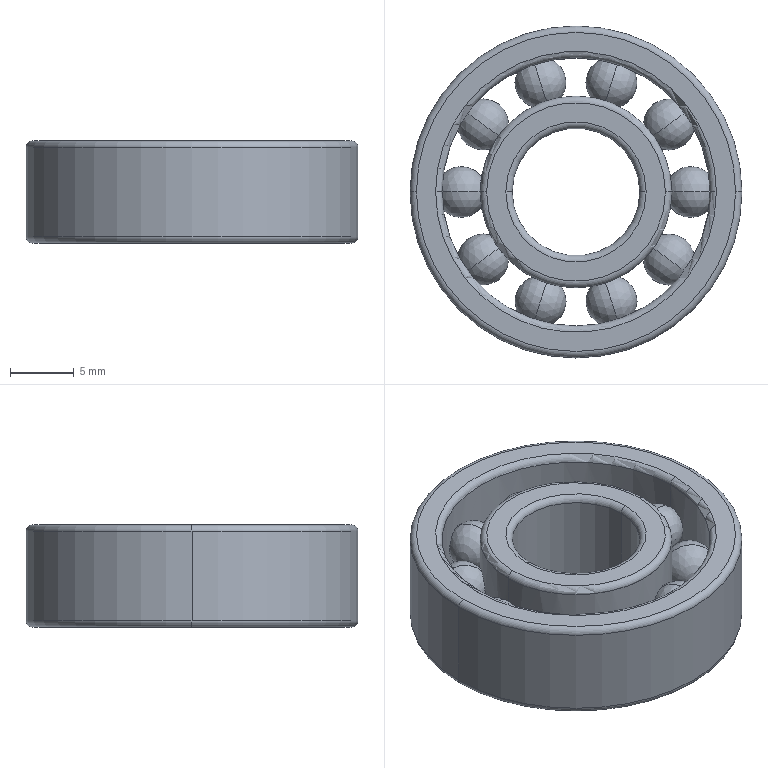Part | STEP file | Bearing 6000Z_P5_BONA_eco | 1 solid | 48 faces | box 26 x 26 x 8 mm | volume 2544 mm3 | sphere 20 | torus 16 | cylinder 8 | plane 4 | commonest cylinder face diameters 10 x2 15 x2 21 x2 26 x2